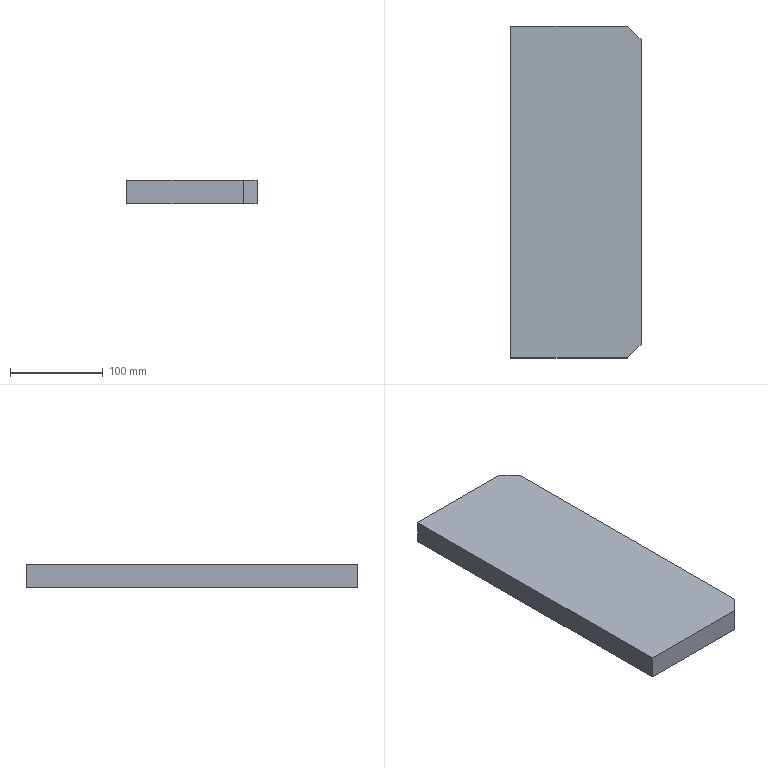Part | SolidWorks | features Chamfer 1, Extrusion 1 | 1 solid | 8 faces | box 140 x 357 x 25 mm | volume 1243875 mm3 | plane 8
STEP:
#1=CARTESIAN_POINT('',(0.,357.,0.));
#2=VERTEX_POINT('',#1);
#3=CARTESIAN_POINT('',(0.,0.,0.));
#4=VERTEX_POINT('',#3);
#5=CARTESIAN_POINT('',(0.,0.,0.));
#6=DIRECTION('',(0.,-1.,0.));
#7=VECTOR('',#6,1000.);
#8=LINE('',#5,#7);
#9=EDGE_CURVE('',#2,#4,#8,.T.);
#10=ORIENTED_EDGE('',*,*,#9,.T.);
#11=CARTESIAN_POINT('',(0.,0.,25.));
#12=VERTEX_POINT('',#11);
#13=CARTESIAN_POINT('',(0.,0.,25.));
#14=DIRECTION('',(0.,0.,-1.));
#15=VECTOR('',#14,1000.);
#16=LINE('',#13,#15);
#17=EDGE_CURVE('',#12,#4,#16,.T.);
#18=ORIENTED_EDGE('',*,*,#17,.F.);
#19=CARTESIAN_POINT('',(0.,357.,25.));
#20=VERTEX_POINT('',#19);
#21=CARTESIAN_POINT('',(0.,0.,25.));
#22=DIRECTION('',(0.,-1.,0.));
#23=VECTOR('',#22,1000.);
#24=LINE('',#21,#23);
#25=EDGE_CURVE('',#20,#12,#24,.T.);
#26=ORIENTED_EDGE('',*,*,#25,.F.);
#27=CARTESIAN_POINT('',(0.,357.,25.));
#28=DIRECTION('',(0.,0.,-1.));
#29=VECTOR('',#28,1000.);
#30=LINE('',#27,#29);
#31=EDGE_CURVE('',#20,#2,#30,.T.);
#32=ORIENTED_EDGE('',*,*,#31,.T.);
#33=EDGE_LOOP('',(#10,#18,#26,#32));
#34=FACE_OUTER_BOUND('',#33,.T.);
#35=CARTESIAN_POINT('',(0.,0.,25.));
#36=DIRECTION('',(1.,0.,0.));
#37=DIRECTION('',(0.,0.,-1.));
#38=AXIS2_PLACEMENT_3D('',#35,#36,#37);
#39=PLANE('',#38);
#40=ADVANCED_FACE('',(#34),#39,.F.);
#41=CARTESIAN_POINT('',(125.,0.,0.));
#42=VERTEX_POINT('',#41);
#43=CARTESIAN_POINT('',(0.,0.,0.));
#44=DIRECTION('',(1.,0.,0.));
#45=VECTOR('',#44,1000.);
#46=LINE('',#43,#45);
#47=EDGE_CURVE('',#4,#42,#46,.T.);
#48=ORIENTED_EDGE('',*,*,#47,.T.);
#49=CARTESIAN_POINT('',(125.,0.,25.));
#50=VERTEX_POINT('',#49);
#51=CARTESIAN_POINT('',(125.,0.,25.));
#52=DIRECTION('',(0.,0.,1.));
#53=VECTOR('',#52,1000.);
#54=LINE('',#51,#53);
#55=EDGE_CURVE('',#42,#50,#54,.T.);
#56=ORIENTED_EDGE('',*,*,#55,.T.);
#57=CARTESIAN_POINT('',(0.,0.,25.));
#58=DIRECTION('',(1.,0.,0.));
#59=VECTOR('',#58,1000.);
#60=LINE('',#57,#59);
#61=EDGE_CURVE('',#12,#50,#60,.T.);
#62=ORIENTED_EDGE('',*,*,#61,.F.);
#63=ORIENTED_EDGE('',*,*,#17,.T.);
#64=EDGE_LOOP('',(#48,#56,#62,#63));
#65=FACE_OUTER_BOUND('',#64,.T.);
#66=CARTESIAN_POINT('',(0.,0.,25.));
#67=DIRECTION('',(0.,1.,0.));
#68=DIRECTION('',(0.,0.,1.));
#69=AXIS2_PLACEMENT_3D('',#66,#67,#68);
#70=PLANE('',#69);
#71=ADVANCED_FACE('',(#65),#70,.F.);
#72=CARTESIAN_POINT('',(140.,15.,25.));
#73=VERTEX_POINT('',#72);
#74=CARTESIAN_POINT('',(140.,342.,25.));
#75=VERTEX_POINT('',#74);
#76=CARTESIAN_POINT('',(140.,0.,25.));
#77=DIRECTION('',(0.,1.,0.));
#78=VECTOR('',#77,1000.);
#79=LINE('',#76,#78);
#80=EDGE_CURVE('',#73,#75,#79,.T.);
#81=ORIENTED_EDGE('',*,*,#80,.F.);
#82=CARTESIAN_POINT('',(140.,15.,0.));
#83=VERTEX_POINT('',#82);
#84=CARTESIAN_POINT('',(140.,15.,25.));
#85=DIRECTION('',(0.,0.,-1.));
#86=VECTOR('',#85,1000.);
#87=LINE('',#84,#86);
#88=EDGE_CURVE('',#73,#83,#87,.T.);
#89=ORIENTED_EDGE('',*,*,#88,.T.);
#90=CARTESIAN_POINT('',(140.,342.,0.));
#91=VERTEX_POINT('',#90);
#92=CARTESIAN_POINT('',(140.,0.,0.));
#93=DIRECTION('',(0.,1.,0.));
#94=VECTOR('',#93,1000.);
#95=LINE('',#92,#94);
#96=EDGE_CURVE('',#83,#91,#95,.T.);
#97=ORIENTED_EDGE('',*,*,#96,.T.);
#98=CARTESIAN_POINT('',(140.,342.,25.));
#99=DIRECTION('',(0.,0.,1.));
#100=VECTOR('',#99,1000.);
#101=LINE('',#98,#100);
#102=EDGE_CURVE('',#91,#75,#101,.T.);
#103=ORIENTED_EDGE('',*,*,#102,.T.);
#104=EDGE_LOOP('',(#81,#89,#97,#103));
#105=FACE_OUTER_BOUND('',#104,.T.);
#106=CARTESIAN_POINT('',(140.,0.,25.));
#107=DIRECTION('',(-1.,0.,0.));
#108=DIRECTION('',(0.,0.,1.));
#109=AXIS2_PLACEMENT_3D('',#106,#107,#108);
#110=PLANE('',#109);
#111=ADVANCED_FACE('',(#105),#110,.F.);
#112=CARTESIAN_POINT('',(125.,357.,25.));
#113=VERTEX_POINT('',#112);
#114=CARTESIAN_POINT('',(0.,357.,25.));
#115=DIRECTION('',(-1.,0.,0.));
#116=VECTOR('',#115,1000.);
#117=LINE('',#114,#116);
#118=EDGE_CURVE('',#113,#20,#117,.T.);
#119=ORIENTED_EDGE('',*,*,#118,.F.);
#120=CARTESIAN_POINT('',(125.,357.,0.));
#121=VERTEX_POINT('',#120);
#122=CARTESIAN_POINT('',(125.,357.,25.));
#123=DIRECTION('',(0.,0.,-1.));
#124=VECTOR('',#123,1000.);
#125=LINE('',#122,#124);
#126=EDGE_CURVE('',#113,#121,#125,.T.);
#127=ORIENTED_EDGE('',*,*,#126,.T.);
#128=CARTESIAN_POINT('',(0.,357.,0.));
#129=DIRECTION('',(-1.,0.,0.));
#130=VECTOR('',#129,1000.);
#131=LINE('',#128,#130);
#132=EDGE_CURVE('',#121,#2,#131,.T.);
#133=ORIENTED_EDGE('',*,*,#132,.T.);
#134=ORIENTED_EDGE('',*,*,#31,.F.);
#135=EDGE_LOOP('',(#119,#127,#133,#134));
#136=FACE_OUTER_BOUND('',#135,.T.);
#137=CARTESIAN_POINT('',(0.,357.,25.));
#138=DIRECTION('',(0.,-1.,0.));
#139=DIRECTION('',(0.,0.,-1.));
#140=AXIS2_PLACEMENT_3D('',#137,#138,#139);
#141=PLANE('',#140);
#142=ADVANCED_FACE('',(#136),#141,.F.);
#143=ORIENTED_EDGE('',*,*,#61,.T.);
#144=CARTESIAN_POINT('',(140.,15.,25.));
#145=DIRECTION('',(0.7071,0.7071,0.));
#146=VECTOR('',#145,1000.);
#147=LINE('',#144,#146);
#148=EDGE_CURVE('',#50,#73,#147,.T.);
#149=ORIENTED_EDGE('',*,*,#148,.T.);
#150=ORIENTED_EDGE('',*,*,#80,.T.);
#151=CARTESIAN_POINT('',(125.,357.,25.));
#152=DIRECTION('',(-0.7071,0.7071,0.));
#153=VECTOR('',#152,1000.);
#154=LINE('',#151,#153);
#155=EDGE_CURVE('',#75,#113,#154,.T.);
#156=ORIENTED_EDGE('',*,*,#155,.T.);
#157=ORIENTED_EDGE('',*,*,#118,.T.);
#158=ORIENTED_EDGE('',*,*,#25,.T.);
#159=EDGE_LOOP('',(#143,#149,#150,#156,#157,#158));
#160=FACE_OUTER_BOUND('',#159,.T.);
#161=CARTESIAN_POINT('',(0.,0.,25.));
#162=DIRECTION('',(0.,0.,-1.));
#163=DIRECTION('',(-1.,0.,0.));
#164=AXIS2_PLACEMENT_3D('',#161,#162,#163);
#165=PLANE('',#164);
#166=ADVANCED_FACE('',(#160),#165,.F.);
#167=ORIENTED_EDGE('',*,*,#96,.F.);
#168=CARTESIAN_POINT('',(62.5,-62.5,0.));
#169=DIRECTION('',(-0.7071,-0.7071,0.));
#170=VECTOR('',#169,1000.);
#171=LINE('',#168,#170);
#172=EDGE_CURVE('',#83,#42,#171,.T.);
#173=ORIENTED_EDGE('',*,*,#172,.T.);
#174=ORIENTED_EDGE('',*,*,#47,.F.);
#175=ORIENTED_EDGE('',*,*,#9,.F.);
#176=ORIENTED_EDGE('',*,*,#132,.F.);
#177=CARTESIAN_POINT('',(241.,241.,0.));
#178=DIRECTION('',(0.7071,-0.7071,0.));
#179=VECTOR('',#178,1000.);
#180=LINE('',#177,#179);
#181=EDGE_CURVE('',#121,#91,#180,.T.);
#182=ORIENTED_EDGE('',*,*,#181,.T.);
#183=EDGE_LOOP('',(#167,#173,#174,#175,#176,#182));
#184=FACE_OUTER_BOUND('',#183,.T.);
#185=CARTESIAN_POINT('',(0.,0.,0.));
#186=DIRECTION('',(0.,0.,-1.));
#187=DIRECTION('',(-1.,0.,0.));
#188=AXIS2_PLACEMENT_3D('',#185,#186,#187);
#189=PLANE('',#188);
#190=ADVANCED_FACE('',(#184),#189,.T.);
#191=ORIENTED_EDGE('',*,*,#148,.F.);
#192=ORIENTED_EDGE('',*,*,#55,.F.);
#193=ORIENTED_EDGE('',*,*,#172,.F.);
#194=ORIENTED_EDGE('',*,*,#88,.F.);
#195=EDGE_LOOP('',(#191,#192,#193,#194));
#196=FACE_OUTER_BOUND('',#195,.T.);
#197=CARTESIAN_POINT('',(140.,15.,25.));
#198=DIRECTION('',(-0.7071,0.7071,0.));
#199=DIRECTION('',(0.,0.,-1.));
#200=AXIS2_PLACEMENT_3D('',#197,#198,#199);
#201=PLANE('',#200);
#202=ADVANCED_FACE('',(#196),#201,.F.);
#203=ORIENTED_EDGE('',*,*,#155,.F.);
#204=ORIENTED_EDGE('',*,*,#102,.F.);
#205=ORIENTED_EDGE('',*,*,#181,.F.);
#206=ORIENTED_EDGE('',*,*,#126,.F.);
#207=EDGE_LOOP('',(#203,#204,#205,#206));
#208=FACE_OUTER_BOUND('',#207,.T.);
#209=CARTESIAN_POINT('',(125.,357.,25.));
#210=DIRECTION('',(-0.7071,-0.7071,0.));
#211=DIRECTION('',(0.,0.,-1.));
#212=AXIS2_PLACEMENT_3D('',#209,#210,#211);
#213=PLANE('',#212);
#214=ADVANCED_FACE('',(#208),#213,.F.);
#215=CLOSED_SHELL('',(#40,#71,#111,#142,#166,#190,#202,#214));
#216=MANIFOLD_SOLID_BREP('',#215);
#217=CARTESIAN_POINT('',(0.,0.,0.));
#218=DIRECTION('',(0.,0.,1.));
#219=DIRECTION('',(1.,0.,0.));
#220=AXIS2_PLACEMENT_3D('',#217,#218,#219);
#221=(LENGTH_UNIT()NAMED_UNIT(*)SI_UNIT(.MILLI.,.METRE.));
#222=UNCERTAINTY_MEASURE_WITH_UNIT(LENGTH_MEASURE(0.00001),#221,'','');
#223=(NAMED_UNIT(*)PLANE_ANGLE_UNIT()SI_UNIT($,.RADIAN.));
#224=(NAMED_UNIT(*)SI_UNIT($,.STERADIAN.)SOLID_ANGLE_UNIT());
#225=(GEOMETRIC_REPRESENTATION_CONTEXT(3)GLOBAL_UNCERTAINTY_ASSIGNED_CONTEXT((#222))GLOBAL_UNIT_ASSIGNED_CONTEXT((#221,#223,#224))REPRESENTATION_CONTEXT('',''));
#226=ADVANCED_BREP_SHAPE_REPRESENTATION('',(#216,#220),#225);